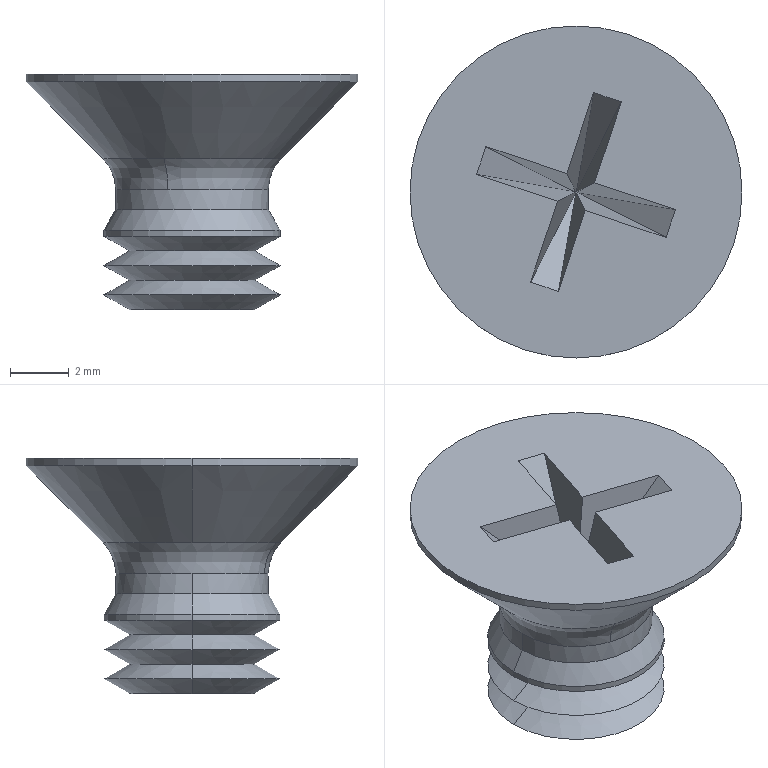Part | SolidWorks | features BaseBody 1 | 1 solid | 36 faces | box 11.3 x 11.3 x 8 mm | volume 284.251 mm3 | cone 14 | plane 14 | cylinder 6 | spline 2 | commonest cylinder face diameters 5.196 x2 6 x2 11.3 x2
STEP:
#1=CARTESIAN_POINT('',(20.376,-44.453,77.752));
#2=VERTEX_POINT('',#1);
#3=CARTESIAN_POINT('',(9.076,-44.453,77.752));
#4=VERTEX_POINT('',#3);
#5=CARTESIAN_POINT('',(14.726,-44.453,77.752));
#6=DIRECTION('',(0.,0.,1.));
#7=DIRECTION('',(1.,0.,0.));
#8=AXIS2_PLACEMENT_3D('',#5,#6,#7);
#9=CIRCLE('',#8,5.65);
#10=EDGE_CURVE('',#2,#4,#9,.T.);
#11=ORIENTED_EDGE('',*,*,#10,.T.);
#12=CARTESIAN_POINT('',(9.076,-44.453,78.));
#13=VERTEX_POINT('',#12);
#14=CARTESIAN_POINT('',(9.076,-44.453,77.752));
#15=DIRECTION('',(0.,0.,1.));
#16=VECTOR('',#15,1000.);
#17=LINE('',#14,#16);
#18=EDGE_CURVE('',#4,#13,#17,.T.);
#19=ORIENTED_EDGE('',*,*,#18,.T.);
#20=CARTESIAN_POINT('',(20.376,-44.453,78.));
#21=VERTEX_POINT('',#20);
#22=CARTESIAN_POINT('',(14.726,-44.453,78.));
#23=DIRECTION('',(0.,0.,1.));
#24=DIRECTION('',(1.,0.,0.));
#25=AXIS2_PLACEMENT_3D('',#22,#23,#24);
#26=CIRCLE('',#25,5.65);
#27=EDGE_CURVE('',#21,#13,#26,.T.);
#28=ORIENTED_EDGE('',*,*,#27,.F.);
#29=CARTESIAN_POINT('',(20.376,-44.453,77.752));
#30=DIRECTION('',(0.,0.,1.));
#31=VECTOR('',#30,1000.);
#32=LINE('',#29,#31);
#33=EDGE_CURVE('',#2,#21,#32,.T.);
#34=ORIENTED_EDGE('',*,*,#33,.F.);
#35=EDGE_LOOP('',(#11,#19,#28,#34));
#36=FACE_OUTER_BOUND('',#35,.T.);
#37=CARTESIAN_POINT('',(14.726,-44.453,77.752));
#38=DIRECTION('',(0.,0.,1.));
#39=DIRECTION('',(1.,0.,0.));
#40=AXIS2_PLACEMENT_3D('',#37,#38,#39);
#41=CYLINDRICAL_SURFACE('',#40,5.65);
#42=ADVANCED_FACE('',(#36),#41,.T.);
#43=CARTESIAN_POINT('',(17.324,-44.453,73.396));
#44=VERTEX_POINT('',#43);
#45=CARTESIAN_POINT('',(12.128,-44.453,73.396));
#46=VERTEX_POINT('',#45);
#47=CARTESIAN_POINT('',(14.726,-44.453,73.396));
#48=DIRECTION('',(0.,0.,1.));
#49=DIRECTION('',(1.,0.,0.));
#50=AXIS2_PLACEMENT_3D('',#47,#48,#49);
#51=CIRCLE('',#50,2.598);
#52=EDGE_CURVE('',#44,#46,#51,.T.);
#53=ORIENTED_EDGE('',*,*,#52,.T.);
#54=CARTESIAN_POINT('',(12.128,-44.453,74.079));
#55=VERTEX_POINT('',#54);
#56=CARTESIAN_POINT('',(12.128,-44.453,73.396));
#57=DIRECTION('',(0.,0.,1.));
#58=VECTOR('',#57,1000.);
#59=LINE('',#56,#58);
#60=EDGE_CURVE('',#46,#55,#59,.T.);
#61=ORIENTED_EDGE('',*,*,#60,.T.);
#62=CARTESIAN_POINT('',(15.547,-41.988,74.079));
#63=VERTEX_POINT('',#62);
#64=CARTESIAN_POINT('',(14.726,-44.453,74.079));
#65=DIRECTION('',(0.,0.,-1.));
#66=DIRECTION('',(0.3159,0.9488,0.));
#67=AXIS2_PLACEMENT_3D('',#64,#65,#66);
#68=CIRCLE('',#67,2.598);
#69=EDGE_CURVE('',#55,#63,#68,.T.);
#70=ORIENTED_EDGE('',*,*,#69,.T.);
#71=CARTESIAN_POINT('',(17.324,-44.453,74.079));
#72=VERTEX_POINT('',#71);
#73=CARTESIAN_POINT('',(14.726,-44.453,74.079));
#74=DIRECTION('',(0.,0.,-1.));
#75=DIRECTION('',(-0.3159,-0.9488,0.));
#76=AXIS2_PLACEMENT_3D('',#73,#74,#75);
#77=CIRCLE('',#76,2.598);
#78=EDGE_CURVE('',#63,#72,#77,.T.);
#79=ORIENTED_EDGE('',*,*,#78,.T.);
#80=CARTESIAN_POINT('',(17.324,-44.453,73.396));
#81=DIRECTION('',(0.,0.,1.));
#82=VECTOR('',#81,1000.);
#83=LINE('',#80,#82);
#84=EDGE_CURVE('',#44,#72,#83,.T.);
#85=ORIENTED_EDGE('',*,*,#84,.F.);
#86=EDGE_LOOP('',(#53,#61,#70,#79,#85));
#87=FACE_OUTER_BOUND('',#86,.T.);
#88=CARTESIAN_POINT('',(14.726,-44.453,73.396));
#89=DIRECTION('',(0.,0.,1.));
#90=DIRECTION('',(1.,0.,0.));
#91=AXIS2_PLACEMENT_3D('',#88,#89,#90);
#92=CYLINDRICAL_SURFACE('',#91,2.598);
#93=ADVANCED_FACE('',(#87),#92,.T.);
#94=ORIENTED_EDGE('',*,*,#52,.F.);
#95=CARTESIAN_POINT('',(17.726,-44.453,72.7));
#96=VERTEX_POINT('',#95);
#97=CARTESIAN_POINT('',(17.726,-44.453,72.7));
#98=DIRECTION('',(0.5,0.,-0.866));
#99=VECTOR('',#98,1000.);
#100=LINE('',#97,#99);
#101=EDGE_CURVE('',#44,#96,#100,.T.);
#102=ORIENTED_EDGE('',*,*,#101,.T.);
#103=CARTESIAN_POINT('',(11.726,-44.453,72.7));
#104=VERTEX_POINT('',#103);
#105=CARTESIAN_POINT('',(14.726,-44.453,72.7));
#106=DIRECTION('',(0.,0.,1.));
#107=DIRECTION('',(-1.,0.,0.));
#108=AXIS2_PLACEMENT_3D('',#105,#106,#107);
#109=CIRCLE('',#108,3.);
#110=EDGE_CURVE('',#96,#104,#109,.T.);
#111=ORIENTED_EDGE('',*,*,#110,.T.);
#112=CARTESIAN_POINT('',(11.726,-44.453,72.7));
#113=DIRECTION('',(-0.5,0.,-0.866));
#114=VECTOR('',#113,1000.);
#115=LINE('',#112,#114);
#116=EDGE_CURVE('',#46,#104,#115,.T.);
#117=ORIENTED_EDGE('',*,*,#116,.F.);
#118=EDGE_LOOP('',(#94,#102,#111,#117));
#119=FACE_OUTER_BOUND('',#118,.T.);
#120=CARTESIAN_POINT('',(14.726,-44.453,72.7));
#121=DIRECTION('',(0.,0.,-1.));
#122=DIRECTION('',(-1.,0.,0.));
#123=AXIS2_PLACEMENT_3D('',#120,#121,#122);
#124=CONICAL_SURFACE('',#123,3.,0.5236);
#125=ADVANCED_FACE('',(#119),#124,.T.);
#126=CARTESIAN_POINT('',(17.726,-44.453,72.495));
#127=VERTEX_POINT('',#126);
#128=CARTESIAN_POINT('',(11.726,-44.453,72.495));
#129=VERTEX_POINT('',#128);
#130=CARTESIAN_POINT('',(14.726,-44.453,72.495));
#131=DIRECTION('',(0.,0.,1.));
#132=DIRECTION('',(1.,0.,0.));
#133=AXIS2_PLACEMENT_3D('',#130,#131,#132);
#134=CIRCLE('',#133,3.);
#135=EDGE_CURVE('',#127,#129,#134,.T.);
#136=ORIENTED_EDGE('',*,*,#135,.T.);
#137=CARTESIAN_POINT('',(11.726,-44.453,72.495));
#138=DIRECTION('',(0.,0.,1.));
#139=VECTOR('',#138,1000.);
#140=LINE('',#137,#139);
#141=EDGE_CURVE('',#129,#104,#140,.T.);
#142=ORIENTED_EDGE('',*,*,#141,.T.);
#143=ORIENTED_EDGE('',*,*,#110,.F.);
#144=CARTESIAN_POINT('',(17.726,-44.453,72.495));
#145=DIRECTION('',(0.,0.,1.));
#146=VECTOR('',#145,1000.);
#147=LINE('',#144,#146);
#148=EDGE_CURVE('',#127,#96,#147,.T.);
#149=ORIENTED_EDGE('',*,*,#148,.F.);
#150=EDGE_LOOP('',(#136,#142,#143,#149));
#151=FACE_OUTER_BOUND('',#150,.T.);
#152=CARTESIAN_POINT('',(14.726,-44.453,72.495));
#153=DIRECTION('',(0.,0.,1.));
#154=DIRECTION('',(1.,0.,0.));
#155=AXIS2_PLACEMENT_3D('',#152,#153,#154);
#156=CYLINDRICAL_SURFACE('',#155,3.);
#157=ADVANCED_FACE('',(#151),#156,.T.);
#158=CARTESIAN_POINT('',(16.86,-44.453,72.));
#159=VERTEX_POINT('',#158);
#160=CARTESIAN_POINT('',(12.592,-44.453,72.));
#161=VERTEX_POINT('',#160);
#162=CARTESIAN_POINT('',(14.726,-44.453,72.));
#163=DIRECTION('',(0.,0.,1.));
#164=DIRECTION('',(0.,-1.,0.));
#165=AXIS2_PLACEMENT_3D('',#162,#163,#164);
#166=CIRCLE('',#165,2.134);
#167=EDGE_CURVE('',#159,#161,#166,.T.);
#168=ORIENTED_EDGE('',*,*,#167,.T.);
#169=CARTESIAN_POINT('',(11.726,-44.453,72.495));
#170=DIRECTION('',(-0.8684,0.,0.4959));
#171=VECTOR('',#170,1000.);
#172=LINE('',#169,#171);
#173=EDGE_CURVE('',#161,#129,#172,.T.);
#174=ORIENTED_EDGE('',*,*,#173,.T.);
#175=ORIENTED_EDGE('',*,*,#135,.F.);
#176=CARTESIAN_POINT('',(17.726,-44.453,72.495));
#177=DIRECTION('',(0.8684,0.,0.4959));
#178=VECTOR('',#177,1000.);
#179=LINE('',#176,#178);
#180=EDGE_CURVE('',#159,#127,#179,.T.);
#181=ORIENTED_EDGE('',*,*,#180,.F.);
#182=EDGE_LOOP('',(#168,#174,#175,#181));
#183=FACE_OUTER_BOUND('',#182,.T.);
#184=CARTESIAN_POINT('',(14.726,-44.453,72.495));
#185=DIRECTION('',(0.,0.,1.));
#186=DIRECTION('',(1.,0.,0.));
#187=AXIS2_PLACEMENT_3D('',#184,#185,#186);
#188=CONICAL_SURFACE('',#187,3.,1.052);
#189=ADVANCED_FACE('',(#183),#188,.T.);
#190=ORIENTED_EDGE('',*,*,#167,.F.);
#191=CARTESIAN_POINT('',(17.726,-44.453,71.495));
#192=VERTEX_POINT('',#191);
#193=CARTESIAN_POINT('',(17.726,-44.453,71.495));
#194=DIRECTION('',(0.8637,0.,-0.5041));
#195=VECTOR('',#194,1000.);
#196=LINE('',#193,#195);
#197=EDGE_CURVE('',#159,#192,#196,.T.);
#198=ORIENTED_EDGE('',*,*,#197,.T.);
#199=CARTESIAN_POINT('',(11.726,-44.453,71.495));
#200=VERTEX_POINT('',#199);
#201=CARTESIAN_POINT('',(14.726,-44.453,71.495));
#202=DIRECTION('',(0.,0.,1.));
#203=DIRECTION('',(0.,1.,0.));
#204=AXIS2_PLACEMENT_3D('',#201,#202,#203);
#205=CIRCLE('',#204,3.);
#206=EDGE_CURVE('',#192,#200,#205,.T.);
#207=ORIENTED_EDGE('',*,*,#206,.T.);
#208=CARTESIAN_POINT('',(11.726,-44.453,71.495));
#209=DIRECTION('',(-0.8637,0.,-0.5041));
#210=VECTOR('',#209,1000.);
#211=LINE('',#208,#210);
#212=EDGE_CURVE('',#161,#200,#211,.T.);
#213=ORIENTED_EDGE('',*,*,#212,.F.);
#214=EDGE_LOOP('',(#190,#198,#207,#213));
#215=FACE_OUTER_BOUND('',#214,.T.);
#216=CARTESIAN_POINT('',(14.726,-44.453,71.495));
#217=DIRECTION('',(0.,0.,-1.));
#218=DIRECTION('',(-1.,0.,0.));
#219=AXIS2_PLACEMENT_3D('',#216,#217,#218);
#220=CONICAL_SURFACE('',#219,3.,1.043);
#221=ADVANCED_FACE('',(#215),#220,.T.);
#222=CARTESIAN_POINT('',(16.86,-44.453,71.));
#223=VERTEX_POINT('',#222);
#224=CARTESIAN_POINT('',(12.592,-44.453,71.));
#225=VERTEX_POINT('',#224);
#226=CARTESIAN_POINT('',(14.726,-44.453,71.));
#227=DIRECTION('',(0.,0.,1.));
#228=DIRECTION('',(1.,0.,0.));
#229=AXIS2_PLACEMENT_3D('',#226,#227,#228);
#230=CIRCLE('',#229,2.134);
#231=EDGE_CURVE('',#223,#225,#230,.T.);
#232=ORIENTED_EDGE('',*,*,#231,.T.);
#233=CARTESIAN_POINT('',(11.726,-44.453,71.495));
#234=DIRECTION('',(-0.8684,0.,0.4959));
#235=VECTOR('',#234,1000.);
#236=LINE('',#233,#235);
#237=EDGE_CURVE('',#225,#200,#236,.T.);
#238=ORIENTED_EDGE('',*,*,#237,.T.);
#239=ORIENTED_EDGE('',*,*,#206,.F.);
#240=CARTESIAN_POINT('',(17.726,-44.453,71.495));
#241=DIRECTION('',(0.8684,0.,0.4959));
#242=VECTOR('',#241,1000.);
#243=LINE('',#240,#242);
#244=EDGE_CURVE('',#223,#192,#243,.T.);
#245=ORIENTED_EDGE('',*,*,#244,.F.);
#246=EDGE_LOOP('',(#232,#238,#239,#245));
#247=FACE_OUTER_BOUND('',#246,.T.);
#248=CARTESIAN_POINT('',(14.726,-44.453,71.495));
#249=DIRECTION('',(0.,0.,1.));
#250=DIRECTION('',(1.,0.,0.));
#251=AXIS2_PLACEMENT_3D('',#248,#249,#250);
#252=CONICAL_SURFACE('',#251,3.,1.052);
#253=ADVANCED_FACE('',(#247),#252,.T.);
#254=ORIENTED_EDGE('',*,*,#231,.F.);
#255=CARTESIAN_POINT('',(17.726,-44.453,70.495));
#256=VERTEX_POINT('',#255);
#257=CARTESIAN_POINT('',(17.726,-44.453,70.495));
#258=DIRECTION('',(0.8637,0.,-0.5041));
#259=VECTOR('',#258,1000.);
#260=LINE('',#257,#259);
#261=EDGE_CURVE('',#223,#256,#260,.T.);
#262=ORIENTED_EDGE('',*,*,#261,.T.);
#263=CARTESIAN_POINT('',(11.726,-44.453,70.495));
#264=VERTEX_POINT('',#263);
#265=CARTESIAN_POINT('',(14.726,-44.453,70.495));
#266=DIRECTION('',(0.,0.,1.));
#267=DIRECTION('',(-1.,0.,0.));
#268=AXIS2_PLACEMENT_3D('',#265,#266,#267);
#269=CIRCLE('',#268,3.);
#270=EDGE_CURVE('',#256,#264,#269,.T.);
#271=ORIENTED_EDGE('',*,*,#270,.T.);
#272=CARTESIAN_POINT('',(11.726,-44.453,70.495));
#273=DIRECTION('',(-0.8637,0.,-0.5041));
#274=VECTOR('',#273,1000.);
#275=LINE('',#272,#274);
#276=EDGE_CURVE('',#225,#264,#275,.T.);
#277=ORIENTED_EDGE('',*,*,#276,.F.);
#278=EDGE_LOOP('',(#254,#262,#271,#277));
#279=FACE_OUTER_BOUND('',#278,.T.);
#280=CARTESIAN_POINT('',(14.726,-44.453,70.495));
#281=DIRECTION('',(0.,0.,-1.));
#282=DIRECTION('',(-1.,0.,0.));
#283=AXIS2_PLACEMENT_3D('',#280,#281,#282);
#284=CONICAL_SURFACE('',#283,3.,1.043);
#285=ADVANCED_FACE('',(#279),#284,.T.);
#286=CARTESIAN_POINT('',(16.86,-44.453,70.));
#287=VERTEX_POINT('',#286);
#288=CARTESIAN_POINT('',(12.592,-44.453,70.));
#289=VERTEX_POINT('',#288);
#290=CARTESIAN_POINT('',(14.726,-44.453,70.));
#291=DIRECTION('',(0.,0.,1.));
#292=DIRECTION('',(1.,0.,0.));
#293=AXIS2_PLACEMENT_3D('',#290,#291,#292);
#294=CIRCLE('',#293,2.134);
#295=EDGE_CURVE('',#287,#289,#294,.T.);
#296=ORIENTED_EDGE('',*,*,#295,.T.);
#297=CARTESIAN_POINT('',(11.726,-44.453,70.495));
#298=DIRECTION('',(-0.8684,0.,0.4959));
#299=VECTOR('',#298,1000.);
#300=LINE('',#297,#299);
#301=EDGE_CURVE('',#289,#264,#300,.T.);
#302=ORIENTED_EDGE('',*,*,#301,.T.);
#303=ORIENTED_EDGE('',*,*,#270,.F.);
#304=CARTESIAN_POINT('',(17.726,-44.453,70.495));
#305=DIRECTION('',(0.8684,0.,0.4959));
#306=VECTOR('',#305,1000.);
#307=LINE('',#304,#306);
#308=EDGE_CURVE('',#287,#256,#307,.T.);
#309=ORIENTED_EDGE('',*,*,#308,.F.);
#310=EDGE_LOOP('',(#296,#302,#303,#309));
#311=FACE_OUTER_BOUND('',#310,.T.);
#312=CARTESIAN_POINT('',(14.726,-44.453,70.495));
#313=DIRECTION('',(0.,0.,1.));
#314=DIRECTION('',(1.,0.,0.));
#315=AXIS2_PLACEMENT_3D('',#312,#313,#314);
#316=CONICAL_SURFACE('',#315,3.,1.052);
#317=ADVANCED_FACE('',(#311),#316,.T.);
#318=CARTESIAN_POINT('',(13.178,-47.521,78.));
#319=VERTEX_POINT('',#318);
#320=CARTESIAN_POINT('',(14.127,-47.837,78.));
#321=VERTEX_POINT('',#320);
#322=CARTESIAN_POINT('',(13.178,-47.521,78.));
#323=DIRECTION('',(0.9488,-0.3159,0.));
#324=VECTOR('',#323,1000.);
#325=LINE('',#322,#324);
#326=EDGE_CURVE('',#319,#321,#325,.T.);
#327=ORIENTED_EDGE('',*,*,#326,.F.);
#328=CARTESIAN_POINT('',(14.094,-44.769,78.));
#329=VERTEX_POINT('',#328);
#330=CARTESIAN_POINT('',(13.178,-47.521,78.));
#331=DIRECTION('',(0.3159,0.9488,0.));
#332=VECTOR('',#331,1000.);
#333=LINE('',#330,#332);
#334=EDGE_CURVE('',#319,#329,#333,.T.);
#335=ORIENTED_EDGE('',*,*,#334,.T.);
#336=CARTESIAN_POINT('',(11.342,-43.853,78.));
#337=VERTEX_POINT('',#336);
#338=CARTESIAN_POINT('',(14.094,-44.769,78.));
#339=DIRECTION('',(-0.9488,0.3159,0.));
#340=VECTOR('',#339,1000.);
#341=LINE('',#338,#340);
#342=EDGE_CURVE('',#329,#337,#341,.T.);
#343=ORIENTED_EDGE('',*,*,#342,.T.);
#344=CARTESIAN_POINT('',(11.658,-42.904,78.));
#345=VERTEX_POINT('',#344);
#346=CARTESIAN_POINT('',(11.658,-42.904,78.));
#347=DIRECTION('',(-0.3159,-0.9488,0.));
#348=VECTOR('',#347,1000.);
#349=LINE('',#346,#348);
#350=EDGE_CURVE('',#345,#337,#349,.T.);
#351=ORIENTED_EDGE('',*,*,#350,.F.);
#352=CARTESIAN_POINT('',(14.41,-43.82,78.));
#353=VERTEX_POINT('',#352);
#354=CARTESIAN_POINT('',(11.658,-42.904,78.));
#355=DIRECTION('',(0.9488,-0.3159,0.));
#356=VECTOR('',#355,1000.);
#357=LINE('',#354,#356);
#358=EDGE_CURVE('',#345,#353,#357,.T.);
#359=ORIENTED_EDGE('',*,*,#358,.T.);
#360=CARTESIAN_POINT('',(15.326,-41.069,78.));
#361=VERTEX_POINT('',#360);
#362=CARTESIAN_POINT('',(14.41,-43.82,78.));
#363=DIRECTION('',(0.3159,0.9488,0.));
#364=VECTOR('',#363,1000.);
#365=LINE('',#362,#364);
#366=EDGE_CURVE('',#353,#361,#365,.T.);
#367=ORIENTED_EDGE('',*,*,#366,.T.);
#368=CARTESIAN_POINT('',(16.274,-41.385,78.));
#369=VERTEX_POINT('',#368);
#370=CARTESIAN_POINT('',(16.274,-41.385,78.));
#371=DIRECTION('',(-0.9488,0.3159,0.));
#372=VECTOR('',#371,1000.);
#373=LINE('',#370,#372);
#374=EDGE_CURVE('',#369,#361,#373,.T.);
#375=ORIENTED_EDGE('',*,*,#374,.F.);
#376=CARTESIAN_POINT('',(15.358,-44.136,78.));
#377=VERTEX_POINT('',#376);
#378=CARTESIAN_POINT('',(16.274,-41.385,78.));
#379=DIRECTION('',(-0.3159,-0.9488,0.));
#380=VECTOR('',#379,1000.);
#381=LINE('',#378,#380);
#382=EDGE_CURVE('',#369,#377,#381,.T.);
#383=ORIENTED_EDGE('',*,*,#382,.T.);
#384=CARTESIAN_POINT('',(18.11,-45.052,78.));
#385=VERTEX_POINT('',#384);
#386=CARTESIAN_POINT('',(15.358,-44.136,78.));
#387=DIRECTION('',(0.9488,-0.3159,0.));
#388=VECTOR('',#387,1000.);
#389=LINE('',#386,#388);
#390=EDGE_CURVE('',#377,#385,#389,.T.);
#391=ORIENTED_EDGE('',*,*,#390,.T.);
#392=CARTESIAN_POINT('',(17.794,-46.001,78.));
#393=VERTEX_POINT('',#392);
#394=CARTESIAN_POINT('',(17.794,-46.001,78.));
#395=DIRECTION('',(0.3159,0.9488,0.));
#396=VECTOR('',#395,1000.);
#397=LINE('',#394,#396);
#398=EDGE_CURVE('',#393,#385,#397,.T.);
#399=ORIENTED_EDGE('',*,*,#398,.F.);
#400=CARTESIAN_POINT('',(15.043,-45.085,78.));
#401=VERTEX_POINT('',#400);
#402=CARTESIAN_POINT('',(17.794,-46.001,78.));
#403=DIRECTION('',(-0.9488,0.3159,0.));
#404=VECTOR('',#403,1000.);
#405=LINE('',#402,#404);
#406=EDGE_CURVE('',#393,#401,#405,.T.);
#407=ORIENTED_EDGE('',*,*,#406,.T.);
#408=CARTESIAN_POINT('',(15.043,-45.085,78.));
#409=DIRECTION('',(-0.3159,-0.9488,0.));
#410=VECTOR('',#409,1000.);
#411=LINE('',#408,#410);
#412=EDGE_CURVE('',#401,#321,#411,.T.);
#413=ORIENTED_EDGE('',*,*,#412,.T.);
#414=EDGE_LOOP('',(#327,#335,#343,#351,#359,#367,#375,#383,#391,#399,#407,#413));
#415=FACE_BOUND('',#414,.T.);
#416=ORIENTED_EDGE('',*,*,#27,.T.);
#417=CARTESIAN_POINT('',(14.726,-44.453,78.));
#418=DIRECTION('',(0.,0.,1.));
#419=DIRECTION('',(1.,0.,0.));
#420=AXIS2_PLACEMENT_3D('',#417,#418,#419);
#421=CIRCLE('',#420,5.65);
#422=EDGE_CURVE('',#13,#21,#421,.T.);
#423=ORIENTED_EDGE('',*,*,#422,.T.);
#424=EDGE_LOOP('',(#416,#423));
#425=FACE_OUTER_BOUND('',#424,.T.);
#426=CARTESIAN_POINT('',(14.726,-44.453,78.));
#427=DIRECTION('',(0.,0.,1.));
#428=DIRECTION('',(1.,0.,0.));
#429=AXIS2_PLACEMENT_3D('',#426,#427,#428);
#430=PLANE('',#429);
#431=ADVANCED_FACE('',(#415,#425),#430,.T.);
#432=ORIENTED_EDGE('',*,*,#334,.F.);
#433=CARTESIAN_POINT('',(14.726,-44.453,74.5));
#434=VERTEX_POINT('',#433);
#435=CARTESIAN_POINT('',(13.178,-47.521,78.));
#436=DIRECTION('',(0.3157,0.6255,-0.7135));
#437=VECTOR('',#436,1000.);
#438=LINE('',#435,#437);
#439=EDGE_CURVE('',#319,#434,#438,.T.);
#440=ORIENTED_EDGE('',*,*,#439,.T.);
#441=CARTESIAN_POINT('',(14.726,-44.453,74.5));
#442=DIRECTION('',(-0.1771,-0.08863,0.9802));
#443=VECTOR('',#442,1000.);
#444=LINE('',#441,#443);
#445=EDGE_CURVE('',#434,#329,#444,.T.);
#446=ORIENTED_EDGE('',*,*,#445,.T.);
#447=EDGE_LOOP('',(#432,#440,#446));
#448=FACE_OUTER_BOUND('',#447,.T.);
#449=CARTESIAN_POINT('',(13.952,-45.987,76.25));
#450=DIRECTION('',(0.9393,-0.3127,0.1414));
#451=DIRECTION('',(0.3159,0.9488,0.));
#452=AXIS2_PLACEMENT_3D('',#449,#450,#451);
#453=PLANE('',#452);
#454=ADVANCED_FACE('',(#448),#453,.T.);
#455=CARTESIAN_POINT('',(14.726,-44.453,74.5));
#456=DIRECTION('',(0.08863,-0.1771,0.9802));
#457=VECTOR('',#456,1000.);
#458=LINE('',#455,#457);
#459=EDGE_CURVE('',#434,#401,#458,.T.);
#460=ORIENTED_EDGE('',*,*,#459,.F.);
#461=CARTESIAN_POINT('',(14.127,-47.837,78.));
#462=DIRECTION('',(0.1222,0.6899,-0.7135));
#463=VECTOR('',#462,1000.);
#464=LINE('',#461,#463);
#465=EDGE_CURVE('',#321,#434,#464,.T.);
#466=ORIENTED_EDGE('',*,*,#465,.F.);
#467=ORIENTED_EDGE('',*,*,#412,.F.);
#468=EDGE_LOOP('',(#460,#466,#467));
#469=FACE_OUTER_BOUND('',#468,.T.);
#470=CARTESIAN_POINT('',(14.426,-46.145,76.25));
#471=DIRECTION('',(0.9393,-0.3127,-0.1414));
#472=DIRECTION('',(0.3159,0.9488,0.));
#473=AXIS2_PLACEMENT_3D('',#470,#471,#472);
#474=PLANE('',#473);
#475=ADVANCED_FACE('',(#469),#474,.F.);
#476=ORIENTED_EDGE('',*,*,#459,.T.);
#477=ORIENTED_EDGE('',*,*,#406,.F.);
#478=CARTESIAN_POINT('',(17.794,-46.001,78.));
#479=DIRECTION('',(-0.6255,0.3157,-0.7135));
#480=VECTOR('',#479,1000.);
#481=LINE('',#478,#480);
#482=EDGE_CURVE('',#393,#434,#481,.T.);
#483=ORIENTED_EDGE('',*,*,#482,.T.);
#484=EDGE_LOOP('',(#476,#477,#483));
#485=FACE_OUTER_BOUND('',#484,.T.);
#486=CARTESIAN_POINT('',(16.26,-45.227,76.25));
#487=DIRECTION('',(0.3127,0.9393,0.1414));
#488=DIRECTION('',(-0.9488,0.3159,0.));
#489=AXIS2_PLACEMENT_3D('',#486,#487,#488);
#490=PLANE('',#489);
#491=ADVANCED_FACE('',(#485),#490,.T.);
#492=ORIENTED_EDGE('',*,*,#390,.F.);
#493=CARTESIAN_POINT('',(14.726,-44.453,74.5));
#494=DIRECTION('',(0.1771,0.08863,0.9802));
#495=VECTOR('',#494,1000.);
#496=LINE('',#493,#495);
#497=EDGE_CURVE('',#434,#377,#496,.T.);
#498=ORIENTED_EDGE('',*,*,#497,.F.);
#499=CARTESIAN_POINT('',(18.11,-45.052,78.));
#500=DIRECTION('',(-0.6899,0.1222,-0.7135));
#501=VECTOR('',#500,1000.);
#502=LINE('',#499,#501);
#503=EDGE_CURVE('',#385,#434,#502,.T.);
#504=ORIENTED_EDGE('',*,*,#503,.F.);
#505=EDGE_LOOP('',(#492,#498,#504));
#506=FACE_OUTER_BOUND('',#505,.T.);
#507=CARTESIAN_POINT('',(16.418,-44.753,76.25));
#508=DIRECTION('',(0.3127,0.9393,-0.1414));
#509=DIRECTION('',(-0.9488,0.3159,0.));
#510=AXIS2_PLACEMENT_3D('',#507,#508,#509);
#511=PLANE('',#510);
#512=ADVANCED_FACE('',(#506),#511,.F.);
#513=ORIENTED_EDGE('',*,*,#497,.T.);
#514=ORIENTED_EDGE('',*,*,#382,.F.);
#515=CARTESIAN_POINT('',(14.726,-44.453,74.5));
#516=DIRECTION('',(0.3157,0.6255,0.7135));
#517=VECTOR('',#516,1000.);
#518=LINE('',#515,#517);
#519=EDGE_CURVE('',#434,#369,#518,.T.);
#520=ORIENTED_EDGE('',*,*,#519,.F.);
#521=EDGE_LOOP('',(#513,#514,#520));
#522=FACE_OUTER_BOUND('',#521,.T.);
#523=CARTESIAN_POINT('',(15.5,-42.919,76.25));
#524=DIRECTION('',(0.9393,-0.3127,-0.1414));
#525=DIRECTION('',(0.3159,0.9488,0.));
#526=AXIS2_PLACEMENT_3D('',#523,#524,#525);
#527=PLANE('',#526);
#528=ADVANCED_FACE('',(#522),#527,.F.);
#529=CARTESIAN_POINT('',(14.726,-44.453,74.5));
#530=DIRECTION('',(0.1222,0.6899,0.7135));
#531=VECTOR('',#530,1000.);
#532=LINE('',#529,#531);
#533=EDGE_CURVE('',#434,#361,#532,.T.);
#534=ORIENTED_EDGE('',*,*,#533,.T.);
#535=ORIENTED_EDGE('',*,*,#366,.F.);
#536=CARTESIAN_POINT('',(14.41,-43.82,78.));
#537=DIRECTION('',(0.08863,-0.1771,-0.9802));
#538=VECTOR('',#537,1000.);
#539=LINE('',#536,#538);
#540=EDGE_CURVE('',#353,#434,#539,.T.);
#541=ORIENTED_EDGE('',*,*,#540,.T.);
#542=EDGE_LOOP('',(#534,#535,#541));
#543=FACE_OUTER_BOUND('',#542,.T.);
#544=CARTESIAN_POINT('',(15.026,-42.761,76.25));
#545=DIRECTION('',(0.9393,-0.3127,0.1414));
#546=DIRECTION('',(0.3159,0.9488,0.));
#547=AXIS2_PLACEMENT_3D('',#544,#545,#546);
#548=PLANE('',#547);
#549=ADVANCED_FACE('',(#543),#548,.T.);
#550=CARTESIAN_POINT('',(14.726,-44.453,74.5));
#551=DIRECTION('',(-0.6255,0.3157,0.7135));
#552=VECTOR('',#551,1000.);
#553=LINE('',#550,#552);
#554=EDGE_CURVE('',#434,#345,#553,.T.);
#555=ORIENTED_EDGE('',*,*,#554,.F.);
#556=ORIENTED_EDGE('',*,*,#540,.F.);
#557=ORIENTED_EDGE('',*,*,#358,.F.);
#558=EDGE_LOOP('',(#555,#556,#557));
#559=FACE_OUTER_BOUND('',#558,.T.);
#560=CARTESIAN_POINT('',(13.192,-43.679,76.25));
#561=DIRECTION('',(0.3127,0.9393,-0.1414));
#562=DIRECTION('',(-0.9488,0.3159,0.));
#563=AXIS2_PLACEMENT_3D('',#560,#561,#562);
#564=PLANE('',#563);
#565=ADVANCED_FACE('',(#559),#564,.F.);
#566=ORIENTED_EDGE('',*,*,#445,.F.);
#567=CARTESIAN_POINT('',(14.726,-44.453,74.5));
#568=DIRECTION('',(-0.6899,0.1222,0.7135));
#569=VECTOR('',#568,1000.);
#570=LINE('',#567,#569);
#571=EDGE_CURVE('',#434,#337,#570,.T.);
#572=ORIENTED_EDGE('',*,*,#571,.T.);
#573=ORIENTED_EDGE('',*,*,#342,.F.);
#574=EDGE_LOOP('',(#566,#572,#573));
#575=FACE_OUTER_BOUND('',#574,.T.);
#576=CARTESIAN_POINT('',(13.034,-44.153,76.25));
#577=DIRECTION('',(0.3127,0.9393,0.1414));
#578=DIRECTION('',(-0.9488,0.3159,0.));
#579=AXIS2_PLACEMENT_3D('',#576,#577,#578);
#580=PLANE('',#579);
#581=ADVANCED_FACE('',(#575),#580,.T.);
#582=ORIENTED_EDGE('',*,*,#18,.F.);
#583=CARTESIAN_POINT('',(14.726,-44.453,77.752));
#584=DIRECTION('',(0.,0.,1.));
#585=DIRECTION('',(1.,0.,0.));
#586=AXIS2_PLACEMENT_3D('',#583,#584,#585);
#587=CIRCLE('',#586,5.65);
#588=EDGE_CURVE('',#4,#2,#587,.T.);
#589=ORIENTED_EDGE('',*,*,#588,.T.);
#590=ORIENTED_EDGE('',*,*,#33,.T.);
#591=ORIENTED_EDGE('',*,*,#422,.F.);
#592=EDGE_LOOP('',(#582,#589,#590,#591));
#593=FACE_OUTER_BOUND('',#592,.T.);
#594=CARTESIAN_POINT('',(14.726,-44.453,77.752));
#595=DIRECTION('',(0.,0.,1.));
#596=DIRECTION('',(1.,0.,0.));
#597=AXIS2_PLACEMENT_3D('',#594,#595,#596);
#598=CYLINDRICAL_SURFACE('',#597,5.65);
#599=ADVANCED_FACE('',(#593),#598,.T.);
#600=ORIENTED_EDGE('',*,*,#465,.T.);
#601=ORIENTED_EDGE('',*,*,#439,.F.);
#602=ORIENTED_EDGE('',*,*,#326,.T.);
#603=EDGE_LOOP('',(#600,#601,#602));
#604=FACE_OUTER_BOUND('',#603,.T.);
#605=CARTESIAN_POINT('',(13.952,-46.068,76.329));
#606=DIRECTION('',(0.2266,0.6806,0.6968));
#607=DIRECTION('',(0.,-0.7154,0.6987));
#608=AXIS2_PLACEMENT_3D('',#605,#606,#607);
#609=PLANE('',#608);
#610=ADVANCED_FACE('',(#604),#609,.T.);
#611=ORIENTED_EDGE('',*,*,#398,.T.);
#612=ORIENTED_EDGE('',*,*,#503,.T.);
#613=ORIENTED_EDGE('',*,*,#482,.F.);
#614=EDGE_LOOP('',(#611,#612,#613));
#615=FACE_OUTER_BOUND('',#614,.T.);
#616=CARTESIAN_POINT('',(16.341,-45.227,76.329));
#617=DIRECTION('',(-0.6806,0.2266,0.6968));
#618=DIRECTION('',(0.7154,0.,0.6987));
#619=AXIS2_PLACEMENT_3D('',#616,#617,#618);
#620=PLANE('',#619);
#621=ADVANCED_FACE('',(#615),#620,.T.);
#622=ORIENTED_EDGE('',*,*,#374,.T.);
#623=ORIENTED_EDGE('',*,*,#533,.F.);
#624=ORIENTED_EDGE('',*,*,#519,.T.);
#625=EDGE_LOOP('',(#622,#623,#624));
#626=FACE_OUTER_BOUND('',#625,.T.);
#627=CARTESIAN_POINT('',(15.5,-42.838,76.329));
#628=DIRECTION('',(-0.2266,-0.6806,0.6968));
#629=DIRECTION('',(0.,-0.7154,-0.6987));
#630=AXIS2_PLACEMENT_3D('',#627,#628,#629);
#631=PLANE('',#630);
#632=ADVANCED_FACE('',(#626),#631,.T.);
#633=ORIENTED_EDGE('',*,*,#571,.F.);
#634=ORIENTED_EDGE('',*,*,#554,.T.);
#635=ORIENTED_EDGE('',*,*,#350,.T.);
#636=EDGE_LOOP('',(#633,#634,#635));
#637=FACE_OUTER_BOUND('',#636,.T.);
#638=CARTESIAN_POINT('',(13.111,-43.679,76.329));
#639=DIRECTION('',(0.6806,-0.2266,0.6968));
#640=DIRECTION('',(0.7154,0.,-0.6987));
#641=AXIS2_PLACEMENT_3D('',#638,#639,#640);
#642=PLANE('',#641);
#643=ADVANCED_FACE('',(#637),#642,.T.);
#644=CARTESIAN_POINT('',(17.763,-44.453,75.139));
#645=VERTEX_POINT('',#644);
#646=CARTESIAN_POINT('',(15.686,-41.571,75.139));
#647=VERTEX_POINT('',#646);
#648=CARTESIAN_POINT('',(14.726,-44.453,75.139));
#649=DIRECTION('',(0.,0.,1.));
#650=DIRECTION('',(1.,0.,0.));
#651=AXIS2_PLACEMENT_3D('',#648,#649,#650);
#652=CIRCLE('',#651,3.037);
#653=EDGE_CURVE('',#645,#647,#652,.T.);
#654=ORIENTED_EDGE('',*,*,#653,.T.);
#655=CARTESIAN_POINT('',(11.689,-44.453,75.139));
#656=VERTEX_POINT('',#655);
#657=CARTESIAN_POINT('',(14.726,-44.453,75.139));
#658=DIRECTION('',(0.,0.,1.));
#659=DIRECTION('',(1.,0.,0.));
#660=AXIS2_PLACEMENT_3D('',#657,#658,#659);
#661=CIRCLE('',#660,3.037);
#662=EDGE_CURVE('',#647,#656,#661,.T.);
#663=ORIENTED_EDGE('',*,*,#662,.T.);
#664=CARTESIAN_POINT('',(-498913.172,-44.453,499000.));
#665=DIRECTION('',(-0.7071,0.,0.7071));
#666=VECTOR('',#665,1000.);
#667=LINE('',#664,#666);
#668=EDGE_CURVE('',#656,#4,#667,.T.);
#669=ORIENTED_EDGE('',*,*,#668,.T.);
#670=ORIENTED_EDGE('',*,*,#10,.F.);
#671=CARTESIAN_POINT('',(498942.624,-44.453,499000.));
#672=DIRECTION('',(-0.7071,0.,-0.7071));
#673=VECTOR('',#672,1000.);
#674=LINE('',#671,#673);
#675=EDGE_CURVE('',#2,#645,#674,.T.);
#676=ORIENTED_EDGE('',*,*,#675,.T.);
#677=EDGE_LOOP('',(#654,#663,#669,#670,#676));
#678=FACE_OUTER_BOUND('',#677,.T.);
#679=CARTESIAN_POINT('',(14.726,-44.453,77.752));
#680=DIRECTION('',(0.,0.,1.));
#681=DIRECTION('',(1.,0.,0.));
#682=AXIS2_PLACEMENT_3D('',#679,#680,#681);
#683=CONICAL_SURFACE('',#682,5.65,0.7854);
#684=ADVANCED_FACE('',(#678),#683,.T.);
#685=ORIENTED_EDGE('',*,*,#588,.F.);
#686=ORIENTED_EDGE('',*,*,#668,.F.);
#687=CARTESIAN_POINT('',(13.767,-47.335,75.139));
#688=VERTEX_POINT('',#687);
#689=CARTESIAN_POINT('',(14.726,-44.453,75.139));
#690=DIRECTION('',(0.,0.,1.));
#691=DIRECTION('',(1.,0.,0.));
#692=AXIS2_PLACEMENT_3D('',#689,#690,#691);
#693=CIRCLE('',#692,3.037);
#694=EDGE_CURVE('',#656,#688,#693,.T.);
#695=ORIENTED_EDGE('',*,*,#694,.T.);
#696=CARTESIAN_POINT('',(14.726,-44.453,75.139));
#697=DIRECTION('',(0.,0.,1.));
#698=DIRECTION('',(1.,0.,0.));
#699=AXIS2_PLACEMENT_3D('',#696,#697,#698);
#700=CIRCLE('',#699,3.037);
#701=EDGE_CURVE('',#688,#645,#700,.T.);
#702=ORIENTED_EDGE('',*,*,#701,.T.);
#703=ORIENTED_EDGE('',*,*,#675,.F.);
#704=EDGE_LOOP('',(#685,#686,#695,#702,#703));
#705=FACE_OUTER_BOUND('',#704,.T.);
#706=CARTESIAN_POINT('',(14.726,-44.453,77.752));
#707=DIRECTION('',(0.,0.,1.));
#708=DIRECTION('',(1.,0.,0.));
#709=AXIS2_PLACEMENT_3D('',#706,#707,#708);
#710=CONICAL_SURFACE('',#709,5.65,0.7854);
#711=ADVANCED_FACE('',(#705),#710,.T.);
#712=ORIENTED_EDGE('',*,*,#694,.F.);
#713=ORIENTED_EDGE('',*,*,#662,.F.);
#714=CARTESIAN_POINT('',(16.021,-40.565,74.079));
#715=DIRECTION('',(-0.9488,0.3159,0.));
#716=DIRECTION('',(0.3159,0.9488,0.));
#717=AXIS2_PLACEMENT_3D('',#714,#715,#716);
#718=CIRCLE('',#717,1.5);
#719=EDGE_CURVE('',#63,#647,#718,.T.);
#720=ORIENTED_EDGE('',*,*,#719,.F.);
#721=ORIENTED_EDGE('',*,*,#69,.F.);
#722=CARTESIAN_POINT('',(13.906,-46.918,74.079));
#723=VERTEX_POINT('',#722);
#724=CARTESIAN_POINT('',(14.726,-44.453,74.079));
#725=DIRECTION('',(0.,0.,-1.));
#726=DIRECTION('',(0.3159,0.9488,0.));
#727=AXIS2_PLACEMENT_3D('',#724,#725,#726);
#728=CIRCLE('',#727,2.598);
#729=EDGE_CURVE('',#723,#55,#728,.T.);
#730=ORIENTED_EDGE('',*,*,#729,.F.);
#731=CARTESIAN_POINT('',(13.432,-48.341,74.079));
#732=DIRECTION('',(-0.9488,0.3159,0.));
#733=DIRECTION('',(-0.3159,-0.9488,0.));
#734=AXIS2_PLACEMENT_3D('',#731,#732,#733);
#735=CIRCLE('',#734,1.5);
#736=EDGE_CURVE('',#688,#723,#735,.T.);
#737=ORIENTED_EDGE('',*,*,#736,.F.);
#738=EDGE_LOOP('',(#712,#713,#720,#721,#730,#737));
#739=FACE_OUTER_BOUND('',#738,.T.);
#740=CARTESIAN_POINT('',(15.547,-41.988,74.079));
#741=CARTESIAN_POINT('',(14.103,-41.507,74.079));
#742=CARTESIAN_POINT('',(12.742,-42.188,74.079));
#743=CARTESIAN_POINT('',(12.261,-43.632,74.079));
#744=CARTESIAN_POINT('',(11.78,-45.076,74.079));
#745=CARTESIAN_POINT('',(12.462,-46.437,74.079));
#746=CARTESIAN_POINT('',(13.906,-46.918,74.079));
#747=CARTESIAN_POINT('',(15.547,-41.988,74.482));
#748=CARTESIAN_POINT('',(14.103,-41.507,74.482));
#749=CARTESIAN_POINT('',(12.742,-42.188,74.482));
#750=CARTESIAN_POINT('',(12.261,-43.632,74.482));
#751=CARTESIAN_POINT('',(11.78,-45.076,74.482));
#752=CARTESIAN_POINT('',(12.462,-46.437,74.482));
#753=CARTESIAN_POINT('',(13.906,-46.918,74.482));
#754=CARTESIAN_POINT('',(15.595,-41.841,74.854));
#755=CARTESIAN_POINT('',(14.066,-41.332,74.854));
#756=CARTESIAN_POINT('',(12.624,-42.054,74.854));
#757=CARTESIAN_POINT('',(12.115,-43.583,74.854));
#758=CARTESIAN_POINT('',(11.606,-45.113,74.854));
#759=CARTESIAN_POINT('',(12.327,-46.555,74.854));
#760=CARTESIAN_POINT('',(13.857,-47.064,74.854));
#761=CARTESIAN_POINT('',(15.686,-41.571,75.139));
#762=CARTESIAN_POINT('',(13.997,-41.009,75.139));
#763=CARTESIAN_POINT('',(12.406,-41.805,75.139));
#764=CARTESIAN_POINT('',(11.844,-43.493,75.139));
#765=CARTESIAN_POINT('',(11.282,-45.182,75.139));
#766=CARTESIAN_POINT('',(12.079,-46.773,75.139));
#767=CARTESIAN_POINT('',(13.767,-47.335,75.139));
#768=(BOUNDED_SURFACE()B_SPLINE_SURFACE(3,3,((#740,#741,#742,#743,#744,#745,#746),(#747,#748,#749,#750,#751,#752,#753),(#754,#755,#756,#757,#758,#759,#760),(#761,#762,#763,#764,#765,#766,#767)),.UNSPECIFIED.,.F.,.F.,.T.)B_SPLINE_SURFACE_WITH_KNOTS((4,4),(4,3,4),(0.,1.),(0.,0.5,1.),.UNSPECIFIED.)GEOMETRIC_REPRESENTATION_ITEM()RATIONAL_B_SPLINE_SURFACE(((1.,0.8047,0.8047,1.,0.8047,0.8047,1.),(0.9493,0.7639,0.7639,0.9493,0.7639,0.7639,0.9493),(0.9493,0.7639,0.7639,0.9493,0.7639,0.7639,0.9493),(1.,0.8047,0.8047,1.,0.8047,0.8047,1.)))REPRESENTATION_ITEM('')SURFACE());
#769=ADVANCED_FACE('',(#739),#768,.F.);
#770=ORIENTED_EDGE('',*,*,#78,.F.);
#771=ORIENTED_EDGE('',*,*,#719,.T.);
#772=ORIENTED_EDGE('',*,*,#653,.F.);
#773=ORIENTED_EDGE('',*,*,#701,.F.);
#774=ORIENTED_EDGE('',*,*,#736,.T.);
#775=CARTESIAN_POINT('',(14.726,-44.453,74.079));
#776=DIRECTION('',(0.,0.,-1.));
#777=DIRECTION('',(-0.3159,-0.9488,0.));
#778=AXIS2_PLACEMENT_3D('',#775,#776,#777);
#779=CIRCLE('',#778,2.598);
#780=EDGE_CURVE('',#72,#723,#779,.T.);
#781=ORIENTED_EDGE('',*,*,#780,.F.);
#782=EDGE_LOOP('',(#770,#771,#772,#773,#774,#781));
#783=FACE_OUTER_BOUND('',#782,.T.);
#784=CARTESIAN_POINT('',(13.906,-46.918,74.079));
#785=CARTESIAN_POINT('',(15.35,-47.398,74.079));
#786=CARTESIAN_POINT('',(16.71,-46.717,74.079));
#787=CARTESIAN_POINT('',(17.191,-45.273,74.079));
#788=CARTESIAN_POINT('',(17.672,-43.829,74.079));
#789=CARTESIAN_POINT('',(16.991,-42.468,74.079));
#790=CARTESIAN_POINT('',(15.547,-41.988,74.079));
#791=CARTESIAN_POINT('',(13.906,-46.918,74.482));
#792=CARTESIAN_POINT('',(15.35,-47.398,74.482));
#793=CARTESIAN_POINT('',(16.71,-46.717,74.482));
#794=CARTESIAN_POINT('',(17.191,-45.273,74.482));
#795=CARTESIAN_POINT('',(17.672,-43.829,74.482));
#796=CARTESIAN_POINT('',(16.991,-42.468,74.482));
#797=CARTESIAN_POINT('',(15.547,-41.988,74.482));
#798=CARTESIAN_POINT('',(13.857,-47.064,74.854));
#799=CARTESIAN_POINT('',(15.387,-47.573,74.854));
#800=CARTESIAN_POINT('',(16.828,-46.852,74.854));
#801=CARTESIAN_POINT('',(17.338,-45.322,74.854));
#802=CARTESIAN_POINT('',(17.847,-43.792,74.854));
#803=CARTESIAN_POINT('',(17.125,-42.351,74.854));
#804=CARTESIAN_POINT('',(15.595,-41.841,74.854));
#805=CARTESIAN_POINT('',(13.767,-47.335,75.139));
#806=CARTESIAN_POINT('',(15.455,-47.897,75.139));
#807=CARTESIAN_POINT('',(17.046,-47.1,75.139));
#808=CARTESIAN_POINT('',(17.608,-45.412,75.139));
#809=CARTESIAN_POINT('',(18.17,-43.724,75.139));
#810=CARTESIAN_POINT('',(17.374,-42.133,75.139));
#811=CARTESIAN_POINT('',(15.686,-41.571,75.139));
#812=(BOUNDED_SURFACE()B_SPLINE_SURFACE(3,3,((#784,#785,#786,#787,#788,#789,#790),(#791,#792,#793,#794,#795,#796,#797),(#798,#799,#800,#801,#802,#803,#804),(#805,#806,#807,#808,#809,#810,#811)),.UNSPECIFIED.,.F.,.F.,.F.)B_SPLINE_SURFACE_WITH_KNOTS((4,4),(4,3,4),(0.,1.),(0.,0.5,1.),.UNSPECIFIED.)GEOMETRIC_REPRESENTATION_ITEM()RATIONAL_B_SPLINE_SURFACE(((1.,0.8047,0.8047,1.,0.8047,0.8047,1.),(0.9493,0.7639,0.7639,0.9493,0.7639,0.7639,0.9493),(0.9493,0.7639,0.7639,0.9493,0.7639,0.7639,0.9493),(1.,0.8047,0.8047,1.,0.8047,0.8047,1.)))REPRESENTATION_ITEM('')SURFACE());
#813=ADVANCED_FACE('',(#783),#812,.F.);
#814=ORIENTED_EDGE('',*,*,#60,.F.);
#815=CARTESIAN_POINT('',(14.726,-44.453,73.396));
#816=DIRECTION('',(0.,0.,1.));
#817=DIRECTION('',(1.,0.,0.));
#818=AXIS2_PLACEMENT_3D('',#815,#816,#817);
#819=CIRCLE('',#818,2.598);
#820=EDGE_CURVE('',#46,#44,#819,.T.);
#821=ORIENTED_EDGE('',*,*,#820,.T.);
#822=ORIENTED_EDGE('',*,*,#84,.T.);
#823=ORIENTED_EDGE('',*,*,#780,.T.);
#824=ORIENTED_EDGE('',*,*,#729,.T.);
#825=EDGE_LOOP('',(#814,#821,#822,#823,#824));
#826=FACE_OUTER_BOUND('',#825,.T.);
#827=CARTESIAN_POINT('',(14.726,-44.453,73.396));
#828=DIRECTION('',(0.,0.,1.));
#829=DIRECTION('',(1.,0.,0.));
#830=AXIS2_PLACEMENT_3D('',#827,#828,#829);
#831=CYLINDRICAL_SURFACE('',#830,2.598);
#832=ADVANCED_FACE('',(#826),#831,.T.);
#833=ORIENTED_EDGE('',*,*,#101,.F.);
#834=ORIENTED_EDGE('',*,*,#820,.F.);
#835=ORIENTED_EDGE('',*,*,#116,.T.);
#836=CARTESIAN_POINT('',(14.726,-44.453,72.7));
#837=DIRECTION('',(0.,0.,1.));
#838=DIRECTION('',(-1.,0.,0.));
#839=AXIS2_PLACEMENT_3D('',#836,#837,#838);
#840=CIRCLE('',#839,3.);
#841=EDGE_CURVE('',#104,#96,#840,.T.);
#842=ORIENTED_EDGE('',*,*,#841,.T.);
#843=EDGE_LOOP('',(#833,#834,#835,#842));
#844=FACE_OUTER_BOUND('',#843,.T.);
#845=CARTESIAN_POINT('',(14.726,-44.453,72.7));
#846=DIRECTION('',(0.,0.,-1.));
#847=DIRECTION('',(-1.,0.,0.));
#848=AXIS2_PLACEMENT_3D('',#845,#846,#847);
#849=CONICAL_SURFACE('',#848,3.,0.5236);
#850=ADVANCED_FACE('',(#844),#849,.T.);
#851=ORIENTED_EDGE('',*,*,#141,.F.);
#852=CARTESIAN_POINT('',(14.726,-44.453,72.495));
#853=DIRECTION('',(0.,0.,1.));
#854=DIRECTION('',(1.,0.,0.));
#855=AXIS2_PLACEMENT_3D('',#852,#853,#854);
#856=CIRCLE('',#855,3.);
#857=EDGE_CURVE('',#129,#127,#856,.T.);
#858=ORIENTED_EDGE('',*,*,#857,.T.);
#859=ORIENTED_EDGE('',*,*,#148,.T.);
#860=ORIENTED_EDGE('',*,*,#841,.F.);
#861=EDGE_LOOP('',(#851,#858,#859,#860));
#862=FACE_OUTER_BOUND('',#861,.T.);
#863=CARTESIAN_POINT('',(14.726,-44.453,72.495));
#864=DIRECTION('',(0.,0.,1.));
#865=DIRECTION('',(1.,0.,0.));
#866=AXIS2_PLACEMENT_3D('',#863,#864,#865);
#867=CYLINDRICAL_SURFACE('',#866,3.);
#868=ADVANCED_FACE('',(#862),#867,.T.);
#869=ORIENTED_EDGE('',*,*,#173,.F.);
#870=CARTESIAN_POINT('',(14.726,-44.453,72.));
#871=DIRECTION('',(0.,0.,1.));
#872=DIRECTION('',(0.,-1.,0.));
#873=AXIS2_PLACEMENT_3D('',#870,#871,#872);
#874=CIRCLE('',#873,2.134);
#875=EDGE_CURVE('',#161,#159,#874,.T.);
#876=ORIENTED_EDGE('',*,*,#875,.T.);
#877=ORIENTED_EDGE('',*,*,#180,.T.);
#878=ORIENTED_EDGE('',*,*,#857,.F.);
#879=EDGE_LOOP('',(#869,#876,#877,#878));
#880=FACE_OUTER_BOUND('',#879,.T.);
#881=CARTESIAN_POINT('',(14.726,-44.453,72.495));
#882=DIRECTION('',(0.,0.,1.));
#883=DIRECTION('',(1.,0.,0.));
#884=AXIS2_PLACEMENT_3D('',#881,#882,#883);
#885=CONICAL_SURFACE('',#884,3.,1.052);
#886=ADVANCED_FACE('',(#880),#885,.T.);
#887=ORIENTED_EDGE('',*,*,#197,.F.);
#888=ORIENTED_EDGE('',*,*,#875,.F.);
#889=ORIENTED_EDGE('',*,*,#212,.T.);
#890=CARTESIAN_POINT('',(14.726,-44.453,71.495));
#891=DIRECTION('',(0.,0.,1.));
#892=DIRECTION('',(0.,1.,0.));
#893=AXIS2_PLACEMENT_3D('',#890,#891,#892);
#894=CIRCLE('',#893,3.);
#895=EDGE_CURVE('',#200,#192,#894,.T.);
#896=ORIENTED_EDGE('',*,*,#895,.T.);
#897=EDGE_LOOP('',(#887,#888,#889,#896));
#898=FACE_OUTER_BOUND('',#897,.T.);
#899=CARTESIAN_POINT('',(14.726,-44.453,71.495));
#900=DIRECTION('',(0.,0.,-1.));
#901=DIRECTION('',(-1.,0.,0.));
#902=AXIS2_PLACEMENT_3D('',#899,#900,#901);
#903=CONICAL_SURFACE('',#902,3.,1.043);
#904=ADVANCED_FACE('',(#898),#903,.T.);
#905=ORIENTED_EDGE('',*,*,#237,.F.);
#906=CARTESIAN_POINT('',(14.726,-44.453,71.));
#907=DIRECTION('',(0.,0.,1.));
#908=DIRECTION('',(1.,0.,0.));
#909=AXIS2_PLACEMENT_3D('',#906,#907,#908);
#910=CIRCLE('',#909,2.134);
#911=EDGE_CURVE('',#225,#223,#910,.T.);
#912=ORIENTED_EDGE('',*,*,#911,.T.);
#913=ORIENTED_EDGE('',*,*,#244,.T.);
#914=ORIENTED_EDGE('',*,*,#895,.F.);
#915=EDGE_LOOP('',(#905,#912,#913,#914));
#916=FACE_OUTER_BOUND('',#915,.T.);
#917=CARTESIAN_POINT('',(14.726,-44.453,71.495));
#918=DIRECTION('',(0.,0.,1.));
#919=DIRECTION('',(1.,0.,0.));
#920=AXIS2_PLACEMENT_3D('',#917,#918,#919);
#921=CONICAL_SURFACE('',#920,3.,1.052);
#922=ADVANCED_FACE('',(#916),#921,.T.);
#923=ORIENTED_EDGE('',*,*,#261,.F.);
#924=ORIENTED_EDGE('',*,*,#911,.F.);
#925=ORIENTED_EDGE('',*,*,#276,.T.);
#926=CARTESIAN_POINT('',(14.726,-44.453,70.495));
#927=DIRECTION('',(0.,0.,1.));
#928=DIRECTION('',(-1.,0.,0.));
#929=AXIS2_PLACEMENT_3D('',#926,#927,#928);
#930=CIRCLE('',#929,3.);
#931=EDGE_CURVE('',#264,#256,#930,.T.);
#932=ORIENTED_EDGE('',*,*,#931,.T.);
#933=EDGE_LOOP('',(#923,#924,#925,#932));
#934=FACE_OUTER_BOUND('',#933,.T.);
#935=CARTESIAN_POINT('',(14.726,-44.453,70.495));
#936=DIRECTION('',(0.,0.,-1.));
#937=DIRECTION('',(-1.,0.,0.));
#938=AXIS2_PLACEMENT_3D('',#935,#936,#937);
#939=CONICAL_SURFACE('',#938,3.,1.043);
#940=ADVANCED_FACE('',(#934),#939,.T.);
#941=ORIENTED_EDGE('',*,*,#301,.F.);
#942=CARTESIAN_POINT('',(14.726,-44.453,70.));
#943=DIRECTION('',(0.,0.,1.));
#944=DIRECTION('',(1.,0.,0.));
#945=AXIS2_PLACEMENT_3D('',#942,#943,#944);
#946=CIRCLE('',#945,2.134);
#947=EDGE_CURVE('',#289,#287,#946,.T.);
#948=ORIENTED_EDGE('',*,*,#947,.T.);
#949=ORIENTED_EDGE('',*,*,#308,.T.);
#950=ORIENTED_EDGE('',*,*,#931,.F.);
#951=EDGE_LOOP('',(#941,#948,#949,#950));
#952=FACE_OUTER_BOUND('',#951,.T.);
#953=CARTESIAN_POINT('',(14.726,-44.453,70.495));
#954=DIRECTION('',(0.,0.,1.));
#955=DIRECTION('',(1.,0.,0.));
#956=AXIS2_PLACEMENT_3D('',#953,#954,#955);
#957=CONICAL_SURFACE('',#956,3.,1.052);
#958=ADVANCED_FACE('',(#952),#957,.T.);
#959=ORIENTED_EDGE('',*,*,#295,.F.);
#960=ORIENTED_EDGE('',*,*,#947,.F.);
#961=EDGE_LOOP('',(#959,#960));
#962=FACE_OUTER_BOUND('',#961,.T.);
#963=CARTESIAN_POINT('',(14.726,-44.453,70.));
#964=DIRECTION('',(0.,0.,1.));
#965=DIRECTION('',(1.,0.,0.));
#966=AXIS2_PLACEMENT_3D('',#963,#964,#965);
#967=PLANE('',#966);
#968=ADVANCED_FACE('',(#962),#967,.F.);
#969=CLOSED_SHELL('',(#42,#93,#125,#157,#189,#221,#253,#285,#317,#431,#454,#475,#491,#512,#528,#549,#565,#581,#599,#610,#621,#632,#643,#684,#711,#769,#813,#832,#850,#868,#886,#904,#922,#940,#958,#968));
#970=MANIFOLD_SOLID_BREP('',#969);
#971=CARTESIAN_POINT('',(0.,0.,0.));
#972=DIRECTION('',(0.,0.,1.));
#973=DIRECTION('',(1.,0.,0.));
#974=AXIS2_PLACEMENT_3D('',#971,#972,#973);
#975=(LENGTH_UNIT()NAMED_UNIT(*)SI_UNIT(.MILLI.,.METRE.));
#976=UNCERTAINTY_MEASURE_WITH_UNIT(LENGTH_MEASURE(0.00001),#975,'','');
#977=(NAMED_UNIT(*)PLANE_ANGLE_UNIT()SI_UNIT($,.RADIAN.));
#978=(NAMED_UNIT(*)SI_UNIT($,.STERADIAN.)SOLID_ANGLE_UNIT());
#979=(GEOMETRIC_REPRESENTATION_CONTEXT(3)GLOBAL_UNCERTAINTY_ASSIGNED_CONTEXT((#976))GLOBAL_UNIT_ASSIGNED_CONTEXT((#975,#977,#978))REPRESENTATION_CONTEXT('',''));
#980=ADVANCED_BREP_SHAPE_REPRESENTATION('',(#970,#974),#979);